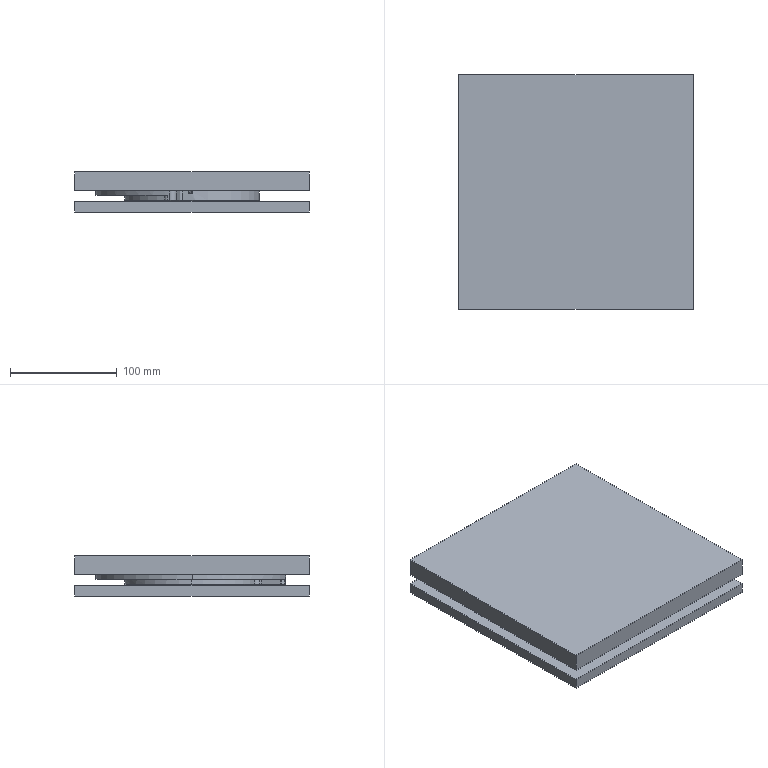CAM job | NX | 3-axis milling, drilling | part box 220 x 220 x 37.5 mm
Tools:
number,name,description,diameter,corner_radius,flute_length,length,flutes
18,D6A45,Milling Tool-5 Parameters,6.0,0.0,3.0,3.0,2
12,2.6ZT,Drilling Tool,2.5,0.0,35.0,50.0,2
13,M3,Milling Tool-5 Parameters,2.5,0.0,30.0,30.0,4
15,5.2ZT,Drilling Tool,5.0,0.0,35.0,50.0,2
16,M6,Milling Tool-5 Parameters,5.0,0.0,30.0,30.0,4
14,4.5ZT,Drilling Tool,4.5,0.0,35.0,50.0,2
3,D10,Milling Tool-5 Parameters,10.0,0.0,50.0,75.0,2
7,D10JING,Milling Tool-5 Parameters,10.0,0.0,50.0,75.0,2
10,D4,Milling Tool-5 Parameters,4.0,0.0,50.0,75.0,2
20,D2,Milling Tool-5 Parameters,2.0,0.0,50.0,75.0,2
9,D6,Milling Tool-5 Parameters,6.0,0.0,50.0,75.0,2
22,D0.5,Milling Tool-5 Parameters,0.5,0.0,50.0,75.0,2
17,3.5ZT,Drilling Tool,3.5,0.0,35.0,50.0,2
Operations:
program,operation,operation_type,tool,method,geometry_group,spindle_rpm,surface_speed,feed_per_tooth,feed_cut,feed_plunge,cut_length_mm,path_length_mm,cut_time_min,machine_time_min
1,DRILLING_COPY_1,Operation,D6A45,METHOD,A,3000.0,56.0,0.0333,200.0,0.0,9.1,91.64,0.0455,0.0538
1,DRILLING_COPY_1_COPY,Operation,D6A45,METHOD,A,3000.0,56.0,0.0333,200.0,0.0,44.8,466.678,0.224,0.2662
1,DRILLING_COPY_1_COPY_1,Operation,2.6ZT,METHOD,A,3000.0,56.0,0.0333,120.0,0.0,22.502,118.445,0.1875,0.1971
1,DRILLING_COPY_1_COPY_1_COPY,Operation,M3,METHOD,A,200.0,1.0,0.0006,0.5,0.0,18.0,109.44,36.0,36.009
1,DRILLING_COPY_1_COPY_1_COPY_1,Operation,5.2ZT,METHOD,A,3000.0,56.0,0.0333,300.0,0.0,108.013,524.219,0.36,0.4017
1,DRILLING_COPY_1_COPY_1_COPY_1_COPY_2,Operation,5.2ZT,METHOD,A,3000.0,56.0,0.0333,300.0,0.0,23.002,106.004,0.0767,0.085
1,DRILLING_COPY_1_COPY_1_COPY_1_COPY,Operation,M6,METHOD,A,200.0,3.0,0.0013,1.0,0.0,93.0,494.193,93.0,93.04
1,DRILLING_COPY_1_COPY_1_COPY_1_COPY_1,Operation,4.5ZT,METHOD,A,3000.0,56.0,0.0333,300.0,0.0,22.852,105.704,0.0762,0.0845
1,ADAPTIVE_MILLING,CavityMilling,D10,METHOD,A,8000.0,251.0,0.2188,3500.0,1000.0,14914.484,21826.815,4.847,5.538
1,ZLEVEL_PROFILE_COPY,ZLevelMilling,D10JING,METHOD,A,8000.0,251.0,0.075,1200.0,100.0,252.086,346.086,0.2101,0.2195
1,ZLEVEL_PROFILE_COPY_1,ZLevelMilling,D6,METHOD,A,9500.0,179.0,0.0789,1500.0,1000.0,1062.599,2251.596,0.7893,0.9082
1,FLOOR_WALL,VolumeBased25DMillingOperation,D6,METHOD,A,9500.0,298.0,0.0526,1000.0,100.0,1463.81,1540.81,1.464,1.472
1,HOLE_MILLING,CylinderMilling,D6,METHOD,A,9500.0,119.0,0.0684,1300.0,100.0,470.696,729.184,0.3621,0.3879
1,ZLEVEL_PROFILE_COPY_1_COPY,ZLevelMilling,D4,METHOD,A,9500.0,179.0,0.0789,1500.0,1000.0,637.572,1242.516,0.4559,0.5164
1,ZLEVEL_PROFILE_COPY_1_COPY_COPY_COPY_COPY_2_COPY,ZLevelMilling,D6A45,METHOD,A,7000.0,131.0,0.0714,1000.0,1000.0,1021.365,1303.01,1.021,1.05
1,ZLEVEL_PROFILE_COPY_2,ZLevelMilling,D2,METHOD,MCS_MILL-A,9500.0,59.0,0.0632,1200.0,1000.0,331.78,386.659,0.2814,0.2869
1,ZLEVEL_PROFILE_COPY_2_COPY,ZLevelMilling,D2,METHOD,MCS_MILL-A,9500.0,59.0,0.0632,1200.0,1000.0,323.378,436.508,0.2793,0.2906
1,ZLEVEL_PROFILE_COPY_2_COPY_COPY,ZLevelMilling,D0.5,METHOD,MCS_MILL-A,9500.0,14.0,0.0526,1000.0,1000.0,1629.242,1738.365,1.629,1.64
1,CUTTERCOMP9,CylinderMilling,D6,METHOD,A,9500.0,119.0,0.0447,850.0,100.0,118.453,376.941,0.1394,0.1652
2夹具,ADAPTIVE_MILLING_COPY,CavityMilling,D10,METHOD,B,8000.0,251.0,0.2188,3500.0,1000.0,24905.756,24966.606,7.519,7.525
2夹具,FLOOR_WALL_COPY,VolumeBased25DMillingOperation,D10JING,METHOD,B,9500.0,298.0,0.0526,1000.0,100.0,3633.077,3704.077,3.633,3.64
2夹具,ZLEVEL_PROFILE_COPY_1_COPY_COPY_COPY_COPY_2_COPY_COPY,ZLevelMilling,D6A45,METHOD,B,7000.0,131.0,0.0714,1000.0,1000.0,535.454,597.454,0.5355,0.5417
2夹具,CUTTERCOMP7,VolumeBased25DMillingOperation,D10JING,METHOD,B,9500.0,298.0,0.0526,1000.0,100.0,514.207,585.207,0.5142,0.5213
3,ADAPTIVE_MILLING_COPY_COPY,CavityMilling,D10,METHOD,C,8000.0,251.0,0.2188,3500.0,1000.0,19748.26,19822.11,5.964,5.971
3,ADAPTIVE_MILLING_COPY_COPY_COPY,CavityMilling,D10,METHOD,C,8000.0,251.0,0.2188,3500.0,1000.0,3022.411,3101.261,1.389,1.397
3,FLOOR_WALL_COPY_COPY,VolumeBased25DMillingOperation,D10JING,METHOD,C,9500.0,298.0,0.0526,1000.0,100.0,2263.66,2656.803,2.264,2.303
3,DRILLING_COPY_1_COPY_2,Operation,D6A45,METHOD,C,3000.0,56.0,0.0333,200.0,0.0,13.65,206.043,0.0683,0.0875
3,DRILLING_COPY_1_COPY_2_COPY,Operation,D6A45,METHOD,C,3000.0,56.0,0.0333,200.0,0.0,29.1,266.546,0.1455,0.1692
3,DRILLING_COPY_1_COPY_1_COPY_2,Operation,2.6ZT,METHOD,C,3000.0,56.0,0.0333,120.0,0.0,29.253,237.25,0.2438,0.2646
3,DRILLING_COPY_1_COPY_1_COPY_COPY,Operation,M3,METHOD,C,200.0,1.0,0.0006,0.5,0.0,27.0,247.743,54.0,54.022
3,DRILLING_COPY_1_COPY_1_COPY_2_COPY,Operation,3.5ZT,METHOD,C,3000.0,56.0,0.0333,120.0,0.0,57.309,322.964,0.4776,0.5041
3,ZLEVEL_PROFILE_COPY_1_COPY_COPY_COPY_COPY_2_COPY_COPY_COPY,ZLevelMilling,D6A45,METHOD,C,7000.0,131.0,0.0714,1000.0,1000.0,669.699,1187.795,0.6697,0.7215
3,ZLEVEL_PROFILE_COPY_1_COPY_COPY_COPY_COPY_2_COPY_COPY_COPY_COPY,ZLevelMilling,D6A45,METHOD,C,7000.0,131.0,0.0714,1000.0,1000.0,429.137,1644.649,0.4291,0.5507
4正面夹具,ADAPTIVE_MILLING_COPY_COPY_COPY_1,CavityMilling,D10,METHOD,D,8000.0,251.0,0.2188,3500.0,1000.0,4882.328,4943.177,1.798,1.804
4正面夹具,FLOOR_WALL_COPY_COPY_COPY,VolumeBased25DMillingOperation,D10JING,METHOD,D,9500.0,298.0,0.0526,1000.0,100.0,868.595,1042.048,0.8686,0.8859
4正面夹具,ZLEVEL_PROFILE_COPY_1_COPY_COPY_COPY_COPY_2_COPY_COPY_COPY_COPY_COPY,ZLevelMilling,D6A45,METHOD,D,7000.0,131.0,0.0714,1000.0,1000.0,229.827,291.827,0.2298,0.236